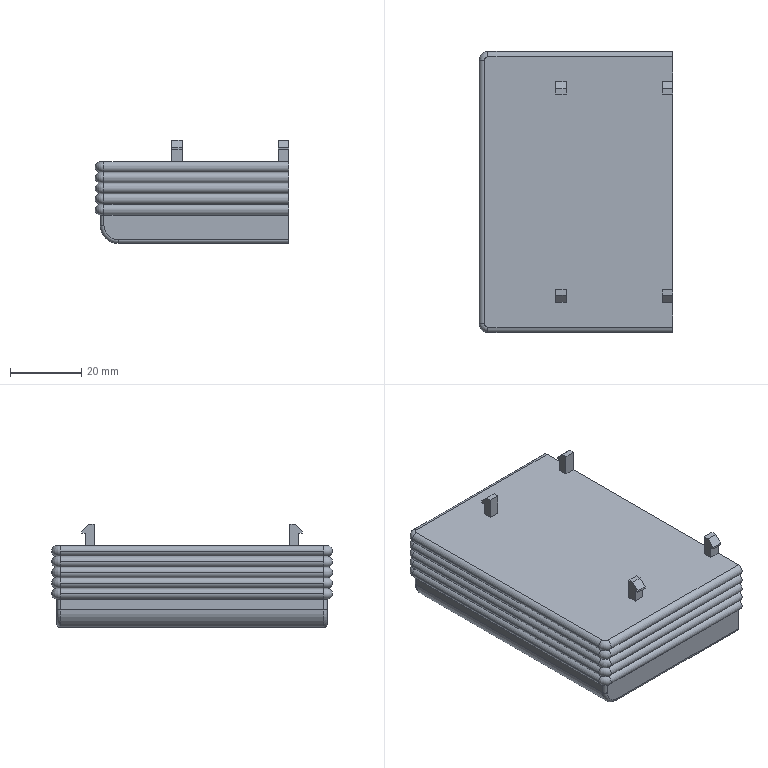Part | SolidWorks | features Chamfer 2, Fillet 2, ICE 2, LPattern 1, MirrorPattern 1, Shell 1, Stock 1, SurfCut 1, Sweep 1 | 1 solid | 84 faces | box 54.5 x 79 x 28.958 mm | volume 25997 mm3 | plane 41 | cylinder 31 | torus 12 | commonest cylinder face diameters 3 x25 2 x4 6 x1 10 x1